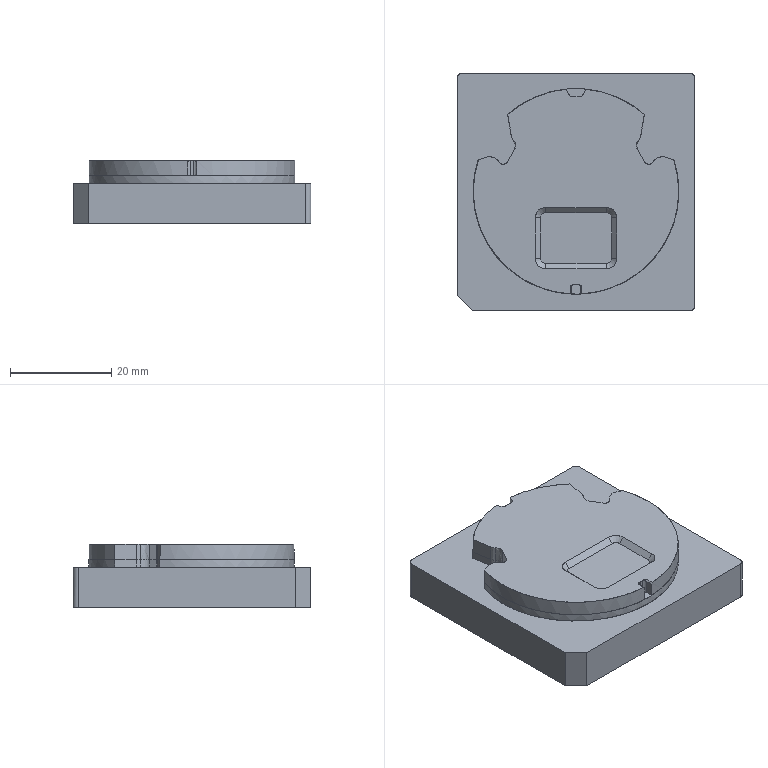NC program | PowerMill | posted with a generic post | part box 47 x 47 x 12.511 mm
Lines 3538 to 4525 of 154620:
N3635 M6
N3636 S18000 M03
N3637 G00 G90 X0.0 Y0.0
N3638 G43 Z9.8015 H15
N3639
N3640 G05 P10000 R4
N3641 X-15.4005 Y12.2096
N3642 Z0.7245
N3643 G01 Z-0.4755 F3000.0
N3644 X-15.382 Y12.2042 F5000.0
N3645 G03 X-15.1667 Y12.3211 I0.0492 J0.1661
N3646 G01 X-14.6715 Y13.9937
N3647 X-14.8477 Y14.9857
N3648 X-14.8683 Y15.4079
N3649 X-14.7556 Y15.83
N3650 X-14.5636 Y16.1357
N3651 X-13.4518 Y17.0964
N3652 X-12.3135 Y17.9407
N3653 X-11.1865 Y18.6675
N3654 X-9.9201 Y19.3764
N3655 X-8.6537 Y19.9776
N3656 X-7.4113 Y20.4735
N3657 X-6.1209 Y20.8972
N3658 X-4.8545 Y21.223
N3659 X-3.5881 Y21.4789
N3660 X-1.8996 Y21.6885
N3661 X-1.4775 Y21.621
N3662 X-1.0553 Y21.3899
N3663 X-0.6689 Y20.8956
N3664 X-0.4258 Y20.3743
N3665 X-0.3705 Y20.3113
N3666 X-0.29 Y20.2877
N3667 X0.2893 Y20.2871
N3668 X0.3699 Y20.3106
N3669 X0.4253 Y20.3737
N3670 X0.6689 Y20.8956
N3671 X0.9736 Y21.3177
N3672 X1.0553 Y21.3899
N3673 X1.4775 Y21.621
N3674 X1.8996 Y21.6885
N3675 X3.166 Y21.5431
N3676 X4.4324 Y21.3138
N3677 X6.126 Y20.8956
N3678 X7.4112 Y20.4735
N3679 X8.6537 Y19.9776
N3680 X9.4115 Y19.6292
N3681 X10.7644 Y18.9161
N3682 X12.0308 Y18.1349
N3683 X13.2972 Y17.2205
N3684 X14.4552 Y16.2521
N3685 X14.5636 Y16.1357
N3686 X14.7511 Y15.83
N3687 X14.8663 Y15.4079
N3688 X14.848 Y14.9857
N3689 X14.1415 Y10.9812
N3690 X13.9872 Y10.3423
N3691 X13.7193 Y9.761
N3692 X13.365 Y9.2743
N3693 X13.3459 Y9.2389
N3694 X13.3369 Y9.1997
N3695 X13.3301 Y9.1387
N3696 X13.3326 Y9.0774
N3697 X13.3488 Y9.0349
N3698 X14.3595 Y7.2578
N3699 G03 X14.5924 Y7.2224 I0.1304 J0.0741
N3700 G01 X14.9857 Y7.5902
N3701 X15.3063 Y7.8095
N3702 X15.83 Y8.062
N3703 X16.3511 Y8.2316
N3704 X17.0964 Y8.3236
N3705 X17.5185 Y8.3033
N3706 X17.9476 Y8.2316
N3707 X18.3628 Y8.1189
N3708 X19.6292 Y7.6594
N3709 X20.0513 Y7.4745
N3710 X20.1704 Y7.3873
N3711 X20.4735 Y7.0615
N3712 X20.6839 Y6.5431
N3713 X21.0382 Y5.2767
N3714 X21.3177 Y3.964
N3715 X21.4402 Y3.166
N3716 X21.5904 Y1.8996
N3717 X21.6601 Y0.2111
N3718 X21.6062 Y-1.4775
N3719 X21.4098 Y-3.166
N3720 X21.181 Y-4.4324
N3721 X20.8655 Y-5.6988
N3722 X20.4735 Y-6.9477
N3723 X20.0513 Y-8.074
N3724 X19.4118 Y-9.498
N3725 X18.7329 Y-10.7644
N3726 X17.9331 Y-12.0308
N3727 X17.0964 Y-13.1885
N3728 X16.3097 Y-14.1415
N3729 X15.4079 Y-15.1119
N3730 X14.6626 Y-15.83
N3731 X13.2972 Y-16.9859
N3732 X12.4529 Y-17.6061
N3733 X11.1865 Y-18.4345
N3734 X10.5848 Y-18.7849
N3735 X9.0759 Y-19.554
N3736 X7.8095 Y-20.0878
N3737 X6.1209 Y-20.6632
N3738 X5.2567 Y-20.8956
N3739 X4.4324 Y-21.0847
N3740 X3.1161 Y-21.3177
N3741 X2.7439 Y-21.3726
N3742 X1.0553 Y-21.518
N3743 X0.6332 Y-21.4631
N3744 X0.3095 Y-21.3177
N3745 X0.084 Y-21.1416
N3746 G03 X-0.1147 Y-21.1533 I-0.0926 J-0.1195
N3747 G01 X-0.3095 Y-21.3177
N3748 X-0.6332 Y-21.4631
N3749 X-1.0553 Y-21.518
N3750 X-2.3217 Y-21.4132
N3751 X-3.5881 Y-21.2427
N3752 X-4.4324 Y-21.0857
N3753 X-5.2567 Y-20.8956
N3754 X-6.1209 Y-20.6625
N3755 X-7.3873 Y-20.2475
N3756 X-8.9115 Y-19.6292
N3757 X-9.9201 Y-19.1383
N3758 X-11.1865 Y-18.4345
N3759 X-11.9702 Y-17.9407
N3760 X-13.2972 Y-16.9875
N3761 X-14.6636 Y-15.83
N3762 X-15.4079 Y-15.112
N3763 X-16.2521 Y-14.2066
N3764 X-17.0964 Y-13.1885
N3765 X-17.9407 Y-12.017
N3766 X-18.7328 Y-10.7644
N3767 X-19.2071 Y-9.8964
N3768 X-19.8047 Y-8.6537
N3769 X-20.3171 Y-7.3873
N3770 X-20.8655 Y-5.6988
N3771 X-21.1812 Y-4.4324
N3772 X-21.4127 Y-3.166
N3773 X-21.5996 Y-1.4775
N3774 X-21.6632 Y0.2111
N3775 X-21.5905 Y1.8996
N3776 X-21.5434 Y2.3217
N3777 X-21.3819 Y3.5881
N3778 X-21.0381 Y5.2767
N3779 X-20.6788 Y6.5431
N3780 X-20.4735 Y7.0615
N3781 X-20.1735 Y7.3873
N3782 X-20.0513 Y7.4745
N3783 X-19.6292 Y7.6594
N3784 X-18.3628 Y8.1189
N3785 X-17.9407 Y8.232
N3786 X-17.5185 Y8.3033
N3787 X-17.0964 Y8.3236
N3788 X-16.3512 Y8.2316
N3789 X-15.83 Y8.062
N3790 X-15.4079 Y7.8632
N3791 X-14.9857 Y7.5902
N3792 X-14.7444 Y7.3873
N3793 X-14.5932 Y7.2341
N3794 G03 X-14.3561 Y7.2653 I0.1068 J0.1054
N3795 G01 X-13.3488 Y9.0348
N3796 X-13.3325 Y9.0774
N3797 X-13.3298 Y9.1229
N3798 X-13.334 Y9.1815
N3799 X-13.346 Y9.239
N3800 X-13.365 Y9.2743
N3801 X-13.7193 Y9.761
N3802 X-13.9893 Y10.3423
N3803 X-14.0979 Y10.7644
N3804 X-14.6715 Y13.9937
N3805 X-15.402 Y12.2148 Z-0.6119
N3806 X-15.3836 Y12.2093
N3807 G03 X-15.1682 Y12.3262 I0.0493 J0.1661
N3808 G01 X-14.674 Y13.9933
N3809 X-14.8499 Y14.9857
N3810 X-14.8704 Y15.4079
N3811 X-14.7571 Y15.83
N3812 X-14.5636 Y16.1381
N3813 X-14.4557 Y16.2521
N3814 X-13.4524 Y17.0964
N3815 X-12.3135 Y17.9407
N3816 X-11.1865 Y18.6675
N3817 X-9.9201 Y19.3764
N3818 X-9.0759 Y19.7813
N3819 X-8.988 Y19.8189
N3820 X-8.6537 Y19.9776
N3821 X-8.0336 Y20.2283
N3822 X-7.4113 Y20.4734
N3823 X-6.7677 Y20.6902
N3824 X-6.1209 Y20.8971
N3825 X-5.4886 Y21.0633
N3826 X-4.8545 Y21.223
N3827 X-3.8995 Y21.4159
N3828 X-3.5881 Y21.4823
N3829 X-1.8996 Y21.6931
N3830 X-1.4775 Y21.622
N3831 X-1.0553 Y21.3907
N3832 X-0.9772 Y21.3177
N3833 X-0.6689 Y20.8956
N3834 X-0.4258 Y20.3743
N3835 X-0.3705 Y20.3113
N3836 X-0.29 Y20.2877
N3837 X0.2893 Y20.2871
N3838 X0.3699 Y20.3106
N3839 X0.4253 Y20.3737
N3840 X0.6689 Y20.8956
N3841 X0.9717 Y21.3177
N3842 X1.0553 Y21.3907
N3843 X1.4775 Y21.622
N3844 X1.8996 Y21.6931
N3845 X2.7443 Y21.5915
N3846 X3.5881 Y21.4823
N3847 X4.2925 Y21.3391
N3848 X4.4324 Y21.3137
N3849 X4.5037 Y21.2961
N3850 X4.8545 Y21.2248
N3851 X6.126 Y20.8956
N3852 X7.4112 Y20.4735
N3853 X8.6537 Y19.9776
N3854 X9.4148 Y19.6292
N3855 X10.7644 Y18.9179
N3856 X12.0308 Y18.1364
N3857 X13.2972 Y17.2222
N3858 X14.4578 Y16.2521
N3859 X14.5636 Y16.1381
N3860 X14.7542 Y15.83
N3861 X14.8688 Y15.4079
N3862 X14.8497 Y14.9857
N3863 X14.4544 Y12.7549
N3864 X14.1414 Y10.9812
N3865 X14.1362 Y10.9597
N3866 X14.1016 Y10.7644
N3867 X13.9895 Y10.3423
N3868 X13.7193 Y9.7587
N3869 X13.3666 Y9.2743
N3870 X13.3475 Y9.2389
N3871 X13.3385 Y9.1998
N3872 X13.3317 Y9.1387
N3873 X13.3342 Y9.0774
N3874 X13.3504 Y9.0349
N3875 X14.3527 Y7.2722
N3876 G03 X14.5824 Y7.2339 I0.1304 J0.0741
N3877 G01 X14.9857 Y7.5902
N3878 X15.3036 Y7.8095
N3879 X15.83 Y8.0629
N3880 X16.2521 Y8.2045
N3881 X16.3453 Y8.2284
N3882 X16.4404 Y8.2426
N3883 X16.6743 Y8.2898
N3884 X17.0964 Y8.3236
N3885 X17.5185 Y8.3058
N3886 X17.9476 Y8.2316
N3887 X18.3628 Y8.1207
N3888 X19.6292 Y7.6607
N3889 X20.0513 Y7.476
N3890 X20.1749 Y7.3873
N3891 X20.4735 Y7.0639
N3892 X20.5323 Y6.9652
N3893 X20.6859 Y6.5431
N3894 X21.0394 Y5.2767
N3895 X21.0713 Y5.1208
N3896 X21.3177 Y3.964
N3897 X21.3848 Y3.5659
N3898 X21.4401 Y3.166
N3899 X21.5348 Y2.3678
N3900 X21.5922 Y1.8996
N3901 X21.663 Y0.2111
N3902 X21.6074 Y-1.4775
N3903 X21.4123 Y-3.166
N3904 X21.181 Y-4.4324
N3905 X20.9718 Y-5.2767
N3906 X20.9626 Y-5.3086
N3907 X20.8654 Y-5.6988
N3908 X20.6727 Y-6.3243
N3909 X20.4734 Y-6.9477
N3910 X20.0893 Y-7.9725
N3911 X20.0513 Y-8.0769
N3912 X19.4132 Y-9.498
N3913 X18.733 Y-10.7644
N3914 X17.9338 Y-12.0308
N3915 X17.0964 Y-13.1885
N3916 X16.3097 Y-14.1415
N3917 X15.4079 Y-15.1119
N3918 X14.663 Y-15.83
N3919 X13.2972 Y-16.9864
N3920 X12.4529 Y-17.6064
N3921 X11.1865 Y-18.4346
N3922 X10.5848 Y-18.7849
N3923 X9.0759 Y-19.554
N3924 X9.0655 Y-19.5583
N3925 X7.8094 Y-20.0877
N3926 X7.5959 Y-20.1619
N3927 X7.3873 Y-20.2492
N3928 X6.7518 Y-20.4491
N3929 X6.1209 Y-20.6631
N3930 X5.9086 Y-20.7183
N3931 X5.6988 Y-20.7825
N3932 X5.0669 Y-20.9396
N3933 X4.4324 Y-21.0859
N3934 X3.1234 Y-21.3177
N3935 X2.7439 Y-21.3732
N3936 X1.0553 Y-21.5205
N3937 X0.6332 Y-21.4946
N3938 X0.1963 Y-21.3177
N3939 X0.1116 Y-21.2622
N3940 G03 X-0.094 Y-21.2407 I-0.1148 J-0.1045
N3941 G01 X-0.2111 Y-21.3279
N3942 X-0.6332 Y-21.4946
N3943 X-1.0553 Y-21.5205
N3944 X-1.4424 Y-21.4859
N3945 X-2.3217 Y-21.4132
N3946 X-2.4461 Y-21.3964
N3947 X-2.4494 Y-21.3962
N3948 X-2.7439 Y-21.3699
N3949 X-3.165 Y-21.2996
N3950 X-3.5881 Y-21.2427
N3951 X-4.3154 Y-21.1074
N3952 X-4.4328 Y-21.0878
N3953 X-4.5482 Y-21.059
N3954 X-5.2567 Y-20.8956
N3955 X-5.9406 Y-20.7111
N3956 X-6.1209 Y-20.6661
N3957 X-7.3873 Y-20.2493
N3958 X-8.9145 Y-19.6292
N3959 X-9.002 Y-19.5851
N3960 X-9.9201 Y-19.1383
N3961 X-10.2509 Y-18.9549
N3962 X-10.5889 Y-18.7849
N3963 X-10.8841 Y-18.6036
N3964 X-11.1865 Y-18.4345
N3965 X-11.8987 Y-17.9857
N3966 X-11.9725 Y-17.9407
N3967 X-13.1547 Y-17.0964
N3968 X-13.2099 Y-17.0501
N3969 X-13.2972 Y-16.9874
N3970 X-14.5151 Y-15.9557
N3971 X-14.6651 Y-15.83
N3972 X-15.4079 Y-15.112
N3973 X-16.2521 Y-14.2066
N3974 X-17.0964 Y-13.1885
N3975 X-17.9407 Y-12.0202
N3976 X-18.7349 Y-10.7644
N3977 X-19.2071 Y-9.8964
N3978 X-19.6292 Y-9.0358
N3979 X-19.8993 Y-8.4241
N3980 X-20.1629 Y-7.8095
N3981 X-20.5338 Y-6.7607
N3982 X-20.8654 Y-5.6988
N3983 X-21.0269 Y-5.0665
N3984 X-21.1811 Y-4.4324
N3985 X-21.3898 Y-3.291
N3986 X-21.4142 Y-3.166
N3987 X-21.6046 Y-1.4775
N3988 X-21.6651 Y0.2111
N3989 X-21.5924 Y1.8996
N3990 X-21.571 Y2.0736
N3991 X-21.5434 Y2.3217
N3992 X-21.4613 Y2.9653
N3993 X-21.3846 Y3.5881
N3994 X-21.0393 Y5.2767
N3995 X-20.8005 Y6.1209
N3996 X-20.7824 Y6.1779
N3997 X-20.6788 Y6.5431
N3998 X-20.5982 Y6.7516
N3999 X-20.5323 Y6.9652
N4000 X-20.4735 Y7.0639
N4001 X-20.176 Y7.3873
N4002 X-20.0513 Y7.476
N4003 X-19.6292 Y7.6607
N4004 X-18.3628 Y8.1207
N4005 X-17.9407 Y8.2323
N4006 X-17.5185 Y8.3058
N4007 X-17.0964 Y8.3236
N4008 X-16.6743 Y8.2898
N4009 X-16.3512 Y8.2316
N4010 X-15.83 Y8.0629
N4011 X-15.4079 Y7.8645
N4012 X-14.9857 Y7.5902
N4013 X-14.7425 Y7.3873
N4014 X-14.5938 Y7.2357
N4015 G03 X-14.3563 Y7.2666 I0.1071 J0.105
N4016 G01 X-13.3504 Y9.0348
N4017 X-13.3341 Y9.0774
N4018 X-13.3314 Y9.1229
N4019 X-13.3356 Y9.1815
N4020 X-13.3476 Y9.239
N4021 X-13.3666 Y9.2743
N4022 X-13.7193 Y9.7587
N4023 X-13.9908 Y10.3423
N4024 X-14.1016 Y10.7644
N4025 X-14.674 Y13.9933
N4026 X-15.4035 Y12.22 Z-0.7484
N4027 X-15.3851 Y12.2146
N4028 G03 X-15.1697 Y12.3314 I0.0493 J0.1661
N4029 G01 X-14.6765 Y13.9928
N4030 X-14.8521 Y14.9857
N4031 X-14.8724 Y15.4079
N4032 X-14.7586 Y15.83
N4033 X-14.5636 Y16.1405
N4034 X-14.46 Y16.2521
N4035 X-13.8412 Y16.7691
N4036 X-13.4524 Y17.0964
N4037 X-13.4279 Y17.1145
N4038 X-13.2972 Y17.2237
N4039 X-12.3135 Y17.9407
N4040 X-11.1865 Y18.6675
N4041 X-9.9201 Y19.3764
N4042 X-9.9056 Y19.3833
N4043 X-9.0758 Y19.7813
N4044 X-8.9907 Y19.8177
N4045 X-8.6537 Y19.9776
N4046 X-7.8095 Y20.3239
N4047 X-7.1774 Y20.5512
N4048 X-6.5431 Y20.772
N4049 X-6.1563 Y20.8839
N4050 X-5.7674 Y20.988
N4051 X-5.2767 Y21.1247
N4052 X-4.4331 Y21.3085
N4053 X-3.5881 Y21.4853
N4054 X-1.8996 Y21.6943
N4055 X-1.4775 Y21.6229
N4056 X-1.0553 Y21.3915
N4057 X-0.9738 Y21.3177
N4058 X-0.6689 Y20.8956
N4059 X-0.4258 Y20.3743
N4060 X-0.3705 Y20.3113
N4061 X-0.29 Y20.2877
N4062 X0.2893 Y20.2871
N4063 X0.3699 Y20.3106
N4064 X0.4253 Y20.3737
N4065 X0.6689 Y20.8956
N4066 X0.9706 Y21.3177
N4067 X1.0553 Y21.3915
N4068 X1.4775 Y21.6229
N4069 X1.8996 Y21.6943
N4070 X2.5585 Y21.6127
N4071 X3.166 Y21.543
N4072 X3.2608 Y21.5258
N4073 X3.5881 Y21.4853
N4074 X4.3951 Y21.3205
N4075 X4.4324 Y21.3137
N4076 X4.4527 Y21.3087
N4077 X4.8545 Y21.2266
N4078 X6.126 Y20.8956
N4079 X7.4113 Y20.4735
N4080 X8.6537 Y19.9776
N4081 X9.418 Y19.6292
N4082 X10.7644 Y18.9197
N4083 X12.0308 Y18.1378
N4084 X13.2972 Y17.2237
N4085 X14.4604 Y16.2521
N4086 X14.5636 Y16.1405
N4087 X14.7574 Y15.83
N4088 X14.8713 Y15.4079
N4089 X14.8514 Y14.9857
N4090 X14.1053 Y10.7644
N4091 X13.9919 Y10.3423
N4092 X13.7193 Y9.7564
N4093 X13.3688 Y9.2751
N4094 X13.3549 Y9.2519
N4095 X13.3455 Y9.2264
N4096 X13.3349 Y9.1798
N4097 X13.3322 Y9.1321
N4098 X13.3327 Y9.1008
N4099 X13.3397 Y9.0703
N4100 X13.3548 Y9.0271
N4101 X14.3457 Y7.2845
N4102 X14.3528 Y7.2731
N4103 X14.361 Y7.2624
N4104 G03 X14.5815 Y7.2348 I0.1222 J0.0818
N4105 G01 X14.9857 Y7.5902
N4106 X15.301 Y7.8095
N4107 X15.83 Y8.0642
N4108 X16.2521 Y8.2045
N4109 X16.3417 Y8.2275
N4110 X16.433 Y8.2416
N4111 X16.6743 Y8.291
N4112 X17.0964 Y8.3236
N4113 X17.5185 Y8.3082
N4114 X17.9476 Y8.2316
N4115 X18.3628 Y8.1224
N4116 X19.6292 Y7.662
N4117 X20.0513 Y7.4775
N4118 X20.1795 Y7.3873
N4119 X20.4735 Y7.0663
N4120 X20.5339 Y6.9652
N4121 X20.6871 Y6.5431
N4122 X21.0406 Y5.2767
N4123 X21.2189 Y4.4335
N4124 X21.3863 Y3.5881
N4125 X21.431 Y3.2251
N4126 X21.4401 Y3.166
N4127 X21.4885 Y2.7578
N4128 X21.594 Y1.8996
N4129 X21.6659 Y0.2111
N4130 X21.6086 Y-1.4775
N4131 X21.4148 Y-3.166
N4132 X21.181 Y-4.4324
N4133 X20.9716 Y-5.2789
N4134 X20.7449 Y-6.1209
N4135 X20.6714 Y-6.3302
N4136 X20.6091 Y-6.5431
N4137 X20.4596 Y-6.9791
N4138 X20.2996 Y-7.4113
N4139 X20.1622 Y-7.8095
N4140 X19.7938 Y-8.6561
N4141 X19.4145 Y-9.498
N4142 X18.7339 Y-10.7644
N4143 X17.9345 Y-12.0308
N4144 X17.0964 Y-13.1885
N4145 X16.3097 Y-14.1415
N4146 X15.4079 Y-15.112
N4147 X15.3754 Y-15.1431
N4148 X14.6629 Y-15.83
N4149 X14.6469 Y-15.8435
N4150 X14.5636 Y-15.9236
N4151 X13.2972 Y-16.9879
N4152 X12.6377 Y-17.47
N4153 X11.9699 Y-17.9407
N4154 X11.1865 Y-18.4346
N4155 X10.7661 Y-18.6799
N4156 X10.3423 Y-18.9193
N4157 X9.0759 Y-19.555
N4158 X8.952 Y-19.606
N4159 X7.8094 Y-20.0877
N4160 X7.6602 Y-20.1386
N4161 X7.3873 Y-20.251
N4162 X6.1209 Y-20.6638
N4163 X5.9086 Y-20.7185
N4164 X5.6988 Y-20.7824
N4165 X5.0667 Y-20.9392
N4166 X4.4324 Y-21.0871
N4167 X3.1306 Y-21.3177
N4168 X2.7439 Y-21.3739
N4169 X1.0553 Y-21.5229
N4170 X0.6332 Y-21.4969
N4171 X0.1921 Y-21.3177
N4172 X0.1084 Y-21.2619
N4173 G03 X-0.094 Y-21.243 I-0.112 J-0.1056
N4174 G01 X-0.2111 Y-21.33
N4175 X-0.6332 Y-21.4969
N4176 X-1.0553 Y-21.5229
N4177 X-1.8339 Y-21.4535
N4178 X-2.3217 Y-21.4131
N4179 X-2.3903 Y-21.4039
N4180 X-2.7439 Y-21.3724
N4181 X-3.165 Y-21.3008
N4182 X-3.5881 Y-21.2426
N4183 X-4.0096 Y-21.1625
N4184 X-4.4324 Y-21.0901
N4185 X-5.2787 Y-20.8868
N4186 X-6.1209 Y-20.6672
N4187 X-7.3873 Y-20.2511
N4188 X-8.9176 Y-19.6292
N4189 X-9.0938 Y-19.5404
N4190 X-9.9201 Y-19.1382
N4191 X-10.2526 Y-18.9548
N4192 X-10.5923 Y-18.7849
N4193 X-11.2868 Y-18.3682
N4194 X-11.9747 Y-17.9407
N4195 X-13.1567 Y-17.0964
N4196 X-13.2277 Y-17.0372
N4197 X-13.2971 Y-16.9874
N4198 X-13.885 Y-16.4894
N4199 X-14.5636 Y-15.9238
N4200 X-14.6352 Y-15.855
N4201 X-14.665 Y-15.83
N4202 X-15.3917 Y-15.1276
N4203 X-15.4079 Y-15.112
N4204 X-16.2521 Y-14.2066
N4205 X-17.0964 Y-13.1885
N4206 X-17.9407 Y-12.0234
N4207 X-18.737 Y-10.7644
N4208 X-19.0784 Y-10.1334
N4209 X-19.4117 Y-9.498
N4210 X-19.5163 Y-9.2649
N4211 X-19.6292 Y-9.0358
N4212 X-19.843 Y-8.5549
N4213 X-20.0492 Y-8.0707
N4214 X-20.1658 Y-7.8095
N4215 X-20.2199 Y-7.6512
N4216 X-20.5618 Y-6.6813
N4217 X-20.8654 Y-5.6988
N4218 X-21.0278 Y-5.0667
N4219 X-21.1811 Y-4.4324
N4220 X-21.3675 Y-3.413
N4221 X-21.4157 Y-3.166
N4222 X-21.6088 Y-1.4775
N4223 X-21.6669 Y0.2111
N4224 X-21.5943 Y1.8996
N4225 X-21.5524 Y2.2405
N4226 X-21.5433 Y2.3217
N4227 X-21.5173 Y2.5258
N4228 X-21.3867 Y3.5881
N4229 X-21.0405 Y5.2767
N4230 X-20.8024 Y6.1209
N4231 X-20.673 Y6.5446
N4232 X-20.5339 Y6.9652
N4233 X-20.4735 Y7.0663
N4234 X-20.1785 Y7.3873
N4235 X-20.0513 Y7.4775
N4236 X-19.6292 Y7.662
N4237 X-18.3628 Y8.1224
N4238 X-17.9407 Y8.2327
N4239 X-17.5185 Y8.3082
N4240 X-17.0964 Y8.3236
N4241 X-16.6743 Y8.291
N4242 X-16.3511 Y8.2316
N4243 X-15.83 Y8.0642
N4244 X-15.708 Y8.0055
N4245 X-15.4079 Y7.8645
N4246 X-15.388 Y7.8516
N4247 X-15.3005 Y7.8095
N4248 X-15.147 Y7.6943
N4249 X-14.9858 Y7.5902
N4250 X-14.7612 Y7.4029
N4251 X-14.7406 Y7.3873
N4252 X-14.5947 Y7.2377
N4253 G03 X-14.3569 Y7.2683 I0.1074 J0.1048
N4254 G01 X-13.352 Y9.0348
N4255 X-13.3357 Y9.0774
N4256 X-13.333 Y9.1229
N4257 X-13.3372 Y9.1815
N4258 X-13.3492 Y9.239
N4259 X-13.3682 Y9.2743
N4260 X-13.7193 Y9.7564
N4261 X-13.9922 Y10.3423
N4262 X-14.1053 Y10.7644
N4263 X-14.6765 Y13.9928
N4264 X-15.4042 Y12.2217 Z-0.8849
N4265 X-15.3857 Y12.2162
N4266 G03 X-15.1703 Y12.333 I0.0493 J0.1661
N4267 G01 X-14.6778 Y13.9926
N4268 X-14.8536 Y14.9857
N4269 X-14.8744 Y15.4079
N4270 X-14.7601 Y15.83
N4271 X-14.5636 Y16.1429
N4272 X-14.4624 Y16.2521
N4273 X-13.5521 Y17.0124
N4274 X-13.3174 Y17.2074
N4275 X-13.0716 Y17.3881
N4276 X-12.3135 Y17.9406
N4277 X-12.243 Y17.9861
N4278 X-12.0308 Y18.1393
N4279 X-11.6062 Y18.3994
N4280 X-11.1865 Y18.6675
N4281 X-11.0826 Y18.7256
N4282 X-10.9868 Y18.7849
N4283 X-9.9201 Y19.3764
N4284 X-9.8914 Y19.39
N4285 X-9.0758 Y19.7812
N4286 X-8.992 Y19.8171
N4287 X-8.6537 Y19.9777
N4288 X-7.8095 Y20.3252
N4289 X-7.4812 Y20.4454
N4290 X-7.1505 Y20.5589
N4291 X-6.5431 Y20.7744
N4292 X-6.3306 Y20.8309
N4293 X-6.1209 Y20.897
N4294 X-5.6976 Y21.0078
N4295 X-5.2767 Y21.127
N4296 X-4.7895 Y21.2344
N4297 X-4.3007 Y21.3348
N4298 X-3.5881 Y21.4865
N4299 X-1.8996 Y21.6954
N4300 X-1.4775 Y21.6239
N4301 X-1.0553 Y21.3923
N4302 X-0.9705 Y21.3177
N4303 X-0.6689 Y20.8956
N4304 X-0.4258 Y20.3743
N4305 X-0.3705 Y20.3113
N4306 X-0.29 Y20.2877
N4307 X0.2893 Y20.2871
N4308 X0.3699 Y20.3106
N4309 X0.4253 Y20.3737
N4310 X0.6689 Y20.8956
N4311 X0.97 Y21.3177
N4312 X1.0553 Y21.3923
N4313 X1.4775 Y21.6239
N4314 X1.8996 Y21.6954
N4315 X2.6954 Y21.597
N4316 X3.166 Y21.5429
N4317 X3.239 Y21.5297
N4318 X3.5881 Y21.4865
N4319 X4.8545 Y21.2284
N4320 X6.126 Y20.8956
N4321 X6.9652 Y20.625
N4322 X7.1867 Y20.5448
N4323 X7.4112 Y20.4734
N4324 X7.8196 Y20.3087
N4325 X8.2316 Y20.1535
N4326 X8.8295 Y19.8984
N4327 X9.4212 Y19.6292
N4328 X10.7644 Y18.9214
N4329 X12.0308 Y18.1393
N4330 X13.2972 Y17.2253
N4331 X14.4624 Y16.2521
N4332 X14.5636 Y16.1429
N4333 X14.7602 Y15.83
N4334 X14.8738 Y15.4079
N4335 X14.8531 Y14.9857
N4336 X14.1066 Y10.7644
N4337 X13.9938 Y10.3423
N4338 X13.7193 Y9.7541
N4339 X13.3649 Y9.2672
N4340 X13.3575 Y9.2546
N4341 X13.3443 Y9.2252
N4342 X13.3378 Y9.1935
N4343 X13.3325 Y9.1354
N4344 X13.3329 Y9.1042
N4345 X13.34 Y9.0737
N4346 X13.3585 Y9.0204
N4347 X14.2429 Y7.4651
N4348 X14.353 Y7.2741
N4349 X14.369 Y7.2515
N4350 X14.389 Y7.2323
N4351 G03 X14.5815 Y7.2348 I0.0949 J0.1107
N4352 G01 X14.926 Y7.5395
N4353 X15.2983 Y7.8095
N4354 X15.83 Y8.0655
N4355 X16.2521 Y8.2046
N4356 X16.3383 Y8.2266
N4357 X16.4262 Y8.2407
N4358 X16.6743 Y8.2923
N4359 X17.0964 Y8.3236
N4360 X17.5185 Y8.31
N4361 X17.9407 Y8.2331
N4362 X17.9441 Y8.2323
N4363 X17.9476 Y8.2316
N4364 X18.0037 Y8.2168
N4365 X18.3628 Y8.1241
N4366 X19.6292 Y7.6634
N4367 X20.0513 Y7.479
N4368 X20.1817 Y7.3873
N4369 X20.4735 Y7.0687
N4370 X20.5353 Y6.9652
N4371 X20.6883 Y6.5431
N4372 X21.0418 Y5.2767
N4373 X21.218 Y4.4331
N4374 X21.3876 Y3.5881
N4375 X21.4373 Y3.1834
N4376 X21.44 Y3.166
N4377 X21.4543 Y3.0458
N4378 X21.5953 Y1.8996
N4379 X21.6687 Y0.2111
N4380 X21.6098 Y-1.4775
N4381 X21.417 Y-3.166
N4382 X21.181 Y-4.4324
N4383 X20.9715 Y-5.2787
N4384 X20.7458 Y-6.1209
N4385 X20.6719 Y-6.3302
N4386 X20.6091 Y-6.543
N4387 X20.4731 Y-6.9401
N4388 X20.3285 Y-7.3341
N4389 X20.165 Y-7.8095
N4390 X20.0736 Y-8.0154
N4391 X20.0512 Y-8.0769
N4392 X19.645 Y-8.9815
N4393 X19.4159 Y-9.498
N4394 X18.7352 Y-10.7644
N4395 X17.9352 Y-12.0308
N4396 X17.0964 Y-13.1885
N4397 X16.3097 Y-14.1415
N4398 X15.4079 Y-15.112
N4399 X15.1419 Y-15.3682
N4400 X14.6629 Y-15.8299
N4401 X14.6603 Y-15.8321
N4402 X14.5636 Y-15.9253
N4403 X13.2972 Y-16.9895
N4404 X12.6376 Y-17.4693
N4405 X11.972 Y-17.9407
N4406 X11.1865 Y-18.4346
N4407 X11.163 Y-18.4482
N4408 X10.5848 Y-18.7848
N4409 X10.5307 Y-18.8124
N4410 X10.3423 Y-18.9209
N4411 X9.892 Y-19.1453
N4412 X9.0758 Y-19.555
N4413 X9.0399 Y-19.5698
N4414 X8.9206 Y-19.6292
N4415 X8.3636 Y-19.8549
N4416 X7.8094 Y-20.0876
N4417 X7.7095 Y-20.1217
N4418 X7.3873 Y-20.2527
N4419 X6.1209 Y-20.6641
N4420 X5.9086 Y-20.7186
N4421 X5.6988 Y-20.7824
N4422 X5.0665 Y-20.939
N4423 X4.4324 Y-21.0883
N4424 X3.1332 Y-21.3177
N4425 X2.7439 Y-21.3745
N4426 X1.0553 Y-21.5246
N4427 X0.6332 Y-21.4993
N4428 X0.1879 Y-21.3177
N4429 X0.1565 Y-21.294
N4430 X0.1084 Y-21.2619
N4431 X0.0907 Y-21.2473
N4432 X0.0744 Y-21.2373
N4433 X0.0002 Y-21.2152
N4434 X-0.0749 Y-21.2338
N4435 X-0.0903 Y-21.2425
N4436 X-0.2111 Y-21.3321
N4437 X-0.6332 Y-21.4993
N4438 X-1.0553 Y-21.5246
N4439 X-2.1893 Y-21.4241
N4440 X-2.3217 Y-21.4131
N4441 X-2.3387 Y-21.4108
N4442 X-2.7439 Y-21.3749
N4443 X-3.3126 Y-21.2797
N4444 X-3.5881 Y-21.2426
N4445 X-4.0096 Y-21.1636
N4446 X-4.4324 Y-21.0922
N4447 X-5.2782 Y-20.886
N4448 X-6.1209 Y-20.668
N4449 X-7.3873 Y-20.2527
N4450 X-8.9206 Y-19.6292
N4451 X-9.7607 Y-19.2129
N4452 X-10.5948 Y-18.7849
N4453 X-10.9888 Y-18.5443
N4454 X-11.1865 Y-18.4344
N4455 X-11.7487 Y-18.0801
N4456 X-11.977 Y-17.9407
N4457 X-13.1588 Y-17.0964
N4458 X-13.4469 Y-16.8628
N4459 X-13.7288 Y-16.6217
N4460 X-14.5636 Y-15.9264
N4461 X-14.6543 Y-15.8389
N4462 X-14.665 Y-15.8299
N4463 X-15.3271 Y-15.19
N4464 X-15.4079 Y-15.112
N4465 X-16.2521 Y-14.2066
N4466 X-17.0964 Y-13.1885
N4467 X-17.9407 Y-12.0266
N4468 X-18.7385 Y-10.7644
N4469 X-18.9237 Y-10.4172
N4470 X-19.207 Y-9.8964
N4471 X-19.6176 Y-9.0595
N4472 X-19.9906 Y-8.2051
N4473 X-20.1671 Y-7.8095
N4474 X-20.3079 Y-7.4098
N4475 G02 X-20.9598 Y-5.3196 I18.6812 J6.9737
N4476 G01 X-21.0495 Y-4.9891
N4477 X-21.0962 Y-4.8169
N4478 X-21.1289 Y-4.6416
N4479 X-21.181 Y-4.4324
N4480 X-21.2952 Y-3.7985
N4481 X-21.4171 Y-3.166
N4482 X-21.61 Y-1.4775
N4483 X-21.6687 Y0.2111
N4484 X-21.5955 Y1.8996
N4485 X-21.3878 Y3.5881
N4486 X-21.0418 Y5.2767
N4487 X-20.6863 Y6.5431
N4488 X-20.5353 Y6.9652
N4489 X-20.4735 Y7.0687
N4490 X-20.181 Y7.3873
N4491 X-20.0513 Y7.479
N4492 X-19.6292 Y7.6634
N4493 X-18.3628 Y8.1241
N4494 X-17.9476 Y8.2316
N4495 X-17.5185 Y8.31
N4496 X-17.0964 Y8.3236
N4497 X-16.6743 Y8.2923
N4498 X-16.3511 Y8.2316
N4499 X-15.83 Y8.0655
N4500 X-15.5914 Y7.9506
N4501 X-15.4079 Y7.8644
N4502 X-15.3955 Y7.8563
N4503 X-15.2981 Y7.8095
N4504 X-15.1458 Y7.6943
N4505 X-14.9858 Y7.5902
N4506 X-14.7803 Y7.4187
N4507 X-14.7387 Y7.3873
N4508 X-14.5945 Y7.2385
N4509 G03 X-14.3569 Y7.2683 I0.1077 J0.104
N4510 G01 X-13.3519 Y9.0348
N4511 X-13.3465 Y9.0469
N4512 X-13.3357 Y9.083
N4513 X-13.3344 Y9.1206
N4514 X-13.3387 Y9.1803
N4515 X-13.351 Y9.2389
N4516 X-13.37 Y9.2741
N4517 X-13.7193 Y9.7541
N4518 X-13.9936 Y10.3423
N4519 X-14.1066 Y10.7644
N4520 X-14.6778 Y13.9926
N4521 X-15.4056 Y12.2209 Z-1.0213
N4522 X-15.3871 Y12.2154
N4523 G03 X-15.1717 Y12.3322 I0.0493 J0.1661
N4524 G01 X-14.679 Y13.9924
N4525 X-14.8548 Y14.9857
N4526 X-14.8757 Y15.4079
N4527 X-14.7616 Y15.83
N4528 X-14.5636 Y16.1452
N4529 X-14.4642 Y16.2521
N4530 X-13.2972 Y17.2268
N4531 X-12.8513 Y17.5486
N4532 X-12.3135 Y17.9406
N4533 X-12.2628 Y17.9733
N4534 X-12.0308 Y18.1407
N4535 X-11.3733 Y18.547
N4536 X-10.8088 Y18.8948
N4537 X-10.2243 Y19.2077
N4538 X-9.6579 Y19.51
N4539 X-9.0758 Y19.7812
N4540 X-8.992 Y19.817
N4541 X-8.6537 Y19.9776
N4542 X-7.876 Y20.2978
N4543 X-7.8095 Y20.3265
N4544 X-7.6089 Y20.396
N4545 X-7.4113 Y20.4733
N4546 X-7.2009 Y20.5424
N4547 X-6.5431 Y20.7757
N4548 X-6.1941 Y20.873
N4549 X-6.074 Y20.9107
N4550 X-5.9517 Y20.9405
N4551 X-5.2767 Y21.1287
N4552 X-5.0646 Y21.1713
N4553 X-4.8545 Y21.2229
N4554 X-4.4408 Y21.3064
N4555 X-3.5881 Y21.4877
N4556 X-1.8996 Y21.6966
N4557 X-1.4775 Y21.6249
N4558 X-1.0553 Y21.3931
N4559 X-0.9693 Y21.3177
N4560 X-0.6689 Y20.8956
N4561 X-0.4258 Y20.3743
N4562 X-0.3705 Y20.3113
N4563 X-0.29 Y20.2877
N4564 X0.2893 Y20.2871
N4565 X0.3699 Y20.3106
N4566 X0.4253 Y20.3737
N4567 X0.6689 Y20.8956
N4568 X0.9693 Y21.3177
N4569 X1.0553 Y21.3931
N4570 X1.4775 Y21.6249
N4571 X1.8996 Y21.6966
N4572 X2.8337 Y21.581
N4573 X3.166 Y21.5429
N4574 X3.2172 Y21.5336
N4575 X3.5881 Y21.4877
N4576 X4.8545 Y21.2302
N4577 X5.7002 Y21.008
N4578 X6.5431 Y20.7757
N4579 X7.1949 Y20.5444
N4580 X7.8084 Y20.3233
N4581 X8.4111 Y20.0744
N4582 X8.6537 Y19.9776
N4583 X9.3056 Y19.6803
N4584 X9.424 Y19.6292
N4585 X10.7644 Y18.9232
N4586 X12.0308 Y18.1407
N4587 X13.2972 Y17.2268
N4588 X14.4642 Y16.2521
N4589 X14.5636 Y16.1452
N4590 X14.7616 Y15.83
N4591 X14.8757 Y15.4079
N4592 X14.8548 Y14.9857
N4593 X14.1078 Y10.7644
N4594 X13.995 Y10.3423
N4595 X13.7193 Y9.7518
N4596 X13.3667 Y9.2668
N4597 X13.34 Y9.2053
N4598 X13.3327 Y9.1387
N4599 X13.3332 Y9.1075
N4600 X13.3402 Y9.077
N4601 X13.3622 Y9.0138
N4602 X14.1371 Y7.6511
N4603 X14.357 Y7.2696
N4604 X14.3649 Y7.2588
N4605 G03 X14.5614 Y7.222 I0.1181 J0.0876
N4606 G01 X14.5816 Y7.2347
N4607 X14.634 Y7.2808
N4608 X14.7369 Y7.3873
N4609 X14.8651 Y7.4841
N4610 X14.9858 Y7.5902
N4611 X15.2323 Y7.7616
N4612 X15.2957 Y7.8095
N4613 X15.83 Y8.0668
N4614 X16.2521 Y8.2046
N4615 X16.3352 Y8.2258
N4616 X16.4198 Y8.2399
N4617 X16.6743 Y8.2935
N4618 X17.0964 Y8.3236
N4619 X17.5185 Y8.3112
N4620 X17.5518 Y8.3039
N4621 X17.9407 Y8.233
N4622 X17.9441 Y8.2322